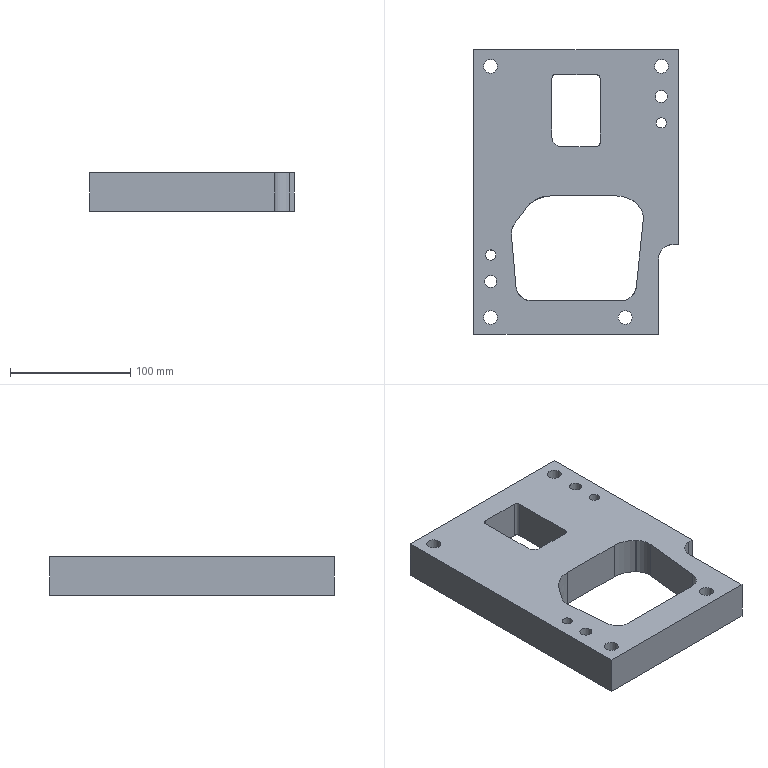Part | STEP file | lll_id3646_x_t | 1 solid | 45 faces | box 170 x 237 x 32 mm | volume 864357 mm3 | plane 22 | cylinder 19 | other 4 | commonest cylinder face diameters 11.509 x4 18.008 x4 6 x3 8.506 x2 10 x2 16 x1
STEP:
#1=CARTESIAN_POINT('',(3672.243,109.5,60.5));
#2=VERTEX_POINT('',#1);
#3=CARTESIAN_POINT('',(3668.,109.5,60.5));
#4=VERTEX_POINT('',#3);
#5=CARTESIAN_POINT('',(3700.5,109.5,60.5));
#6=DIRECTION('',(-1.,0.,0.));
#7=VECTOR('',#6,1.);
#8=LINE('',#5,#7);
#9=EDGE_CURVE('',#2,#4,#8,.T.);
#10=ORIENTED_EDGE('',*,*,#9,.T.);
#11=CARTESIAN_POINT('',(3656.,97.5,60.5));
#12=VERTEX_POINT('',#11);
#13=CARTESIAN_POINT('',(3668.,97.5,60.5));
#14=DIRECTION('',(0.,0.,1.));
#15=DIRECTION('',(-1.,0.,0.));
#16=AXIS2_PLACEMENT_3D('',#13,#14,#15);
#17=CIRCLE('',#16,12.);
#18=EDGE_CURVE('',#4,#12,#17,.T.);
#19=ORIENTED_EDGE('',*,*,#18,.T.);
#20=CARTESIAN_POINT('',(3656.,34.803,60.5));
#21=VERTEX_POINT('',#20);
#22=CARTESIAN_POINT('',(3656.,0.00007612,60.5));
#23=DIRECTION('',(0.,-1.,0.));
#24=VECTOR('',#23,1.);
#25=LINE('',#22,#24);
#26=EDGE_CURVE('',#12,#21,#25,.T.);
#27=ORIENTED_EDGE('',*,*,#26,.T.);
#28=CARTESIAN_POINT('',(3502.243,34.803,60.5));
#29=VERTEX_POINT('',#28);
#30=CARTESIAN_POINT('',(3587.243,34.803,60.5));
#31=DIRECTION('',(1.,0.,0.));
#32=VECTOR('',#31,1.);
#33=LINE('',#30,#32);
#34=EDGE_CURVE('',#29,#21,#33,.T.);
#35=ORIENTED_EDGE('',*,*,#34,.F.);
#36=CARTESIAN_POINT('',(3502.243,271.803,60.5));
#37=VERTEX_POINT('',#36);
#38=CARTESIAN_POINT('',(3502.243,156.803,60.5));
#39=DIRECTION('',(0.,-1.,0.));
#40=VECTOR('',#39,1.);
#41=LINE('',#38,#40);
#42=EDGE_CURVE('',#37,#29,#41,.T.);
#43=ORIENTED_EDGE('',*,*,#42,.F.);
#44=CARTESIAN_POINT('',(3672.243,271.803,60.5));
#45=VERTEX_POINT('',#44);
#46=CARTESIAN_POINT('',(3587.243,271.803,60.5));
#47=DIRECTION('',(-1.,0.,0.));
#48=VECTOR('',#47,1.);
#49=LINE('',#46,#48);
#50=EDGE_CURVE('',#45,#37,#49,.T.);
#51=ORIENTED_EDGE('',*,*,#50,.F.);
#52=CARTESIAN_POINT('',(3672.243,156.803,60.5));
#53=DIRECTION('',(0.,1.,0.));
#54=VECTOR('',#53,1.);
#55=LINE('',#52,#54);
#56=EDGE_CURVE('',#2,#45,#55,.T.);
#57=ORIENTED_EDGE('',*,*,#56,.F.);
#58=EDGE_LOOP('',(#10,#19,#27,#35,#43,#51,#57));
#59=FACE_BOUND('',#58,.T.);
#60=CARTESIAN_POINT('',(3511.99,100.803,60.5));
#61=VERTEX_POINT('',#60);
#62=CARTESIAN_POINT('',(3516.243,100.803,60.5));
#63=DIRECTION('',(0.,0.,1.));
#64=DIRECTION('',(-1.,0.,0.));
#65=AXIS2_PLACEMENT_3D('',#62,#63,#64);
#66=CIRCLE('',#65,4.253);
#67=EDGE_CURVE('',#61,#61,#66,.T.);
#68=ORIENTED_EDGE('',*,*,#67,.T.);
#69=EDGE_LOOP('',(#68));
#70=FACE_BOUND('',#69,.T.);
#71=CARTESIAN_POINT('',(3521.244,78.803,60.5));
#72=VERTEX_POINT('',#71);
#73=CARTESIAN_POINT('',(3516.243,78.803,60.5));
#74=DIRECTION('',(0.,0.,-1.));
#75=DIRECTION('',(1.,0.,0.));
#76=AXIS2_PLACEMENT_3D('',#73,#74,#75);
#77=CIRCLE('',#76,5.);
#78=EDGE_CURVE('',#72,#72,#77,.T.);
#79=ORIENTED_EDGE('',*,*,#78,.F.);
#80=EDGE_LOOP('',(#79));
#81=FACE_BOUND('',#80,.T.);
#82=CARTESIAN_POINT('',(3663.244,232.803,60.5));
#83=VERTEX_POINT('',#82);
#84=CARTESIAN_POINT('',(3658.243,232.803,60.5));
#85=DIRECTION('',(0.,0.,-1.));
#86=DIRECTION('',(1.,0.,0.));
#87=AXIS2_PLACEMENT_3D('',#84,#85,#86);
#88=CIRCLE('',#87,5.);
#89=EDGE_CURVE('',#83,#83,#88,.T.);
#90=ORIENTED_EDGE('',*,*,#89,.F.);
#91=EDGE_LOOP('',(#90));
#92=FACE_BOUND('',#91,.T.);
#93=CARTESIAN_POINT('',(3507.239,257.803,60.5));
#94=VERTEX_POINT('',#93);
#95=CARTESIAN_POINT('',(3516.243,257.803,60.5));
#96=DIRECTION('',(0.,0.,1.));
#97=DIRECTION('',(-1.,0.,0.));
#98=AXIS2_PLACEMENT_3D('',#95,#96,#97);
#99=CIRCLE('',#98,9.004);
#100=EDGE_CURVE('',#94,#94,#99,.T.);
#101=ORIENTED_EDGE('',*,*,#100,.T.);
#102=EDGE_LOOP('',(#101));
#103=FACE_BOUND('',#102,.T.);
#104=CARTESIAN_POINT('',(3649.239,257.803,60.5));
#105=VERTEX_POINT('',#104);
#106=CARTESIAN_POINT('',(3658.243,257.803,60.5));
#107=DIRECTION('',(0.,0.,1.));
#108=DIRECTION('',(-1.,0.,0.));
#109=AXIS2_PLACEMENT_3D('',#106,#107,#108);
#110=CIRCLE('',#109,9.004);
#111=EDGE_CURVE('',#105,#105,#110,.T.);
#112=ORIENTED_EDGE('',*,*,#111,.T.);
#113=EDGE_LOOP('',(#112));
#114=FACE_BOUND('',#113,.T.);
#115=CARTESIAN_POINT('',(3507.239,48.803,60.5));
#116=VERTEX_POINT('',#115);
#117=CARTESIAN_POINT('',(3516.243,48.803,60.5));
#118=DIRECTION('',(0.,0.,1.));
#119=DIRECTION('',(-1.,0.,0.));
#120=AXIS2_PLACEMENT_3D('',#117,#118,#119);
#121=CIRCLE('',#120,9.004);
#122=EDGE_CURVE('',#116,#116,#121,.T.);
#123=ORIENTED_EDGE('',*,*,#122,.T.);
#124=EDGE_LOOP('',(#123));
#125=FACE_BOUND('',#124,.T.);
#126=CARTESIAN_POINT('',(3619.239,48.803,60.5));
#127=VERTEX_POINT('',#126);
#128=CARTESIAN_POINT('',(3628.243,48.803,60.5));
#129=DIRECTION('',(0.,0.,1.));
#130=DIRECTION('',(-1.,0.,0.));
#131=AXIS2_PLACEMENT_3D('',#128,#129,#130);
#132=CIRCLE('',#131,9.004);
#133=EDGE_CURVE('',#127,#127,#132,.T.);
#134=ORIENTED_EDGE('',*,*,#133,.T.);
#135=EDGE_LOOP('',(#134));
#136=FACE_BOUND('',#135,.T.);
#137=CARTESIAN_POINT('',(3653.99,210.803,60.5));
#138=VERTEX_POINT('',#137);
#139=CARTESIAN_POINT('',(3658.243,210.803,60.5));
#140=DIRECTION('',(0.,0.,1.));
#141=DIRECTION('',(-1.,0.,0.));
#142=AXIS2_PLACEMENT_3D('',#139,#140,#141);
#143=CIRCLE('',#142,4.253);
#144=EDGE_CURVE('',#138,#138,#143,.T.);
#145=ORIENTED_EDGE('',*,*,#144,.T.);
#146=EDGE_LOOP('',(#145));
#147=FACE_BOUND('',#146,.T.);
#148=CARTESIAN_POINT('',(3567.234,198.95,60.5));
#149=VERTEX_POINT('',#148);
#150=CARTESIAN_POINT('',(3567.234,247.95,60.5));
#151=VERTEX_POINT('',#150);
#152=CARTESIAN_POINT('',(3567.234,199.225,60.5));
#153=DIRECTION('',(0.,1.,0.));
#154=VECTOR('',#153,1.);
#155=LINE('',#152,#154);
#156=EDGE_CURVE('',#149,#151,#155,.T.);
#157=ORIENTED_EDGE('',*,*,#156,.F.);
#158=CARTESIAN_POINT('',(3575.234,190.95,60.5));
#159=VERTEX_POINT('',#158);
#160=CARTESIAN_POINT('',(3575.234,198.95,60.5));
#161=DIRECTION('',(0.,0.,1.));
#162=DIRECTION('',(1.,0.,0.));
#163=AXIS2_PLACEMENT_3D('',#160,#161,#162);
#164=CIRCLE('',#163,8.);
#165=EDGE_CURVE('',#149,#159,#164,.T.);
#166=ORIENTED_EDGE('',*,*,#165,.T.);
#167=CARTESIAN_POINT('',(3604.234,190.95,60.5));
#168=VERTEX_POINT('',#167);
#169=CARTESIAN_POINT('',(3587.234,190.95,60.5));
#170=DIRECTION('',(-1.,0.,0.));
#171=VECTOR('',#170,1.);
#172=LINE('',#169,#171);
#173=EDGE_CURVE('',#168,#159,#172,.T.);
#174=ORIENTED_EDGE('',*,*,#173,.F.);
#175=CARTESIAN_POINT('',(3607.234,193.95,60.5));
#176=VERTEX_POINT('',#175);
#177=CARTESIAN_POINT('',(3604.234,193.95,60.5));
#178=DIRECTION('',(0.,0.,1.));
#179=DIRECTION('',(1.,0.,0.));
#180=AXIS2_PLACEMENT_3D('',#177,#178,#179);
#181=CIRCLE('',#180,3.);
#182=EDGE_CURVE('',#168,#176,#181,.T.);
#183=ORIENTED_EDGE('',*,*,#182,.T.);
#184=CARTESIAN_POINT('',(3607.234,247.95,60.5));
#185=VERTEX_POINT('',#184);
#186=CARTESIAN_POINT('',(3607.234,199.225,60.5));
#187=DIRECTION('',(0.,-1.,0.));
#188=VECTOR('',#187,1.);
#189=LINE('',#186,#188);
#190=EDGE_CURVE('',#185,#176,#189,.T.);
#191=ORIENTED_EDGE('',*,*,#190,.F.);
#192=CARTESIAN_POINT('',(3604.234,250.95,60.5));
#193=VERTEX_POINT('',#192);
#194=CARTESIAN_POINT('',(3604.234,247.95,60.5));
#195=DIRECTION('',(0.,0.,1.));
#196=DIRECTION('',(1.,0.,0.));
#197=AXIS2_PLACEMENT_3D('',#194,#195,#196);
#198=CIRCLE('',#197,3.);
#199=EDGE_CURVE('',#185,#193,#198,.T.);
#200=ORIENTED_EDGE('',*,*,#199,.T.);
#201=CARTESIAN_POINT('',(3570.234,250.95,60.5));
#202=VERTEX_POINT('',#201);
#203=CARTESIAN_POINT('',(3587.234,250.95,60.5));
#204=DIRECTION('',(1.,0.,0.));
#205=VECTOR('',#204,1.);
#206=LINE('',#203,#205);
#207=EDGE_CURVE('',#202,#193,#206,.T.);
#208=ORIENTED_EDGE('',*,*,#207,.F.);
#209=CARTESIAN_POINT('',(3570.234,247.95,60.5));
#210=DIRECTION('',(0.,0.,1.));
#211=DIRECTION('',(1.,0.,0.));
#212=AXIS2_PLACEMENT_3D('',#209,#210,#211);
#213=CIRCLE('',#212,3.);
#214=EDGE_CURVE('',#202,#151,#213,.T.);
#215=ORIENTED_EDGE('',*,*,#214,.T.);
#216=EDGE_LOOP('',(#157,#166,#174,#183,#191,#200,#208,#215));
#217=FACE_BOUND('',#216,.T.);
#218=CARTESIAN_POINT('',(3620.83,150.017,60.5));
#219=VERTEX_POINT('',#218);
#220=CARTESIAN_POINT('',(3638.507,142.694,60.5));
#221=VERTEX_POINT('',#220);
#222=CARTESIAN_POINT('',(3620.83,125.017,60.5));
#223=DIRECTION('',(0.,0.,-1.));
#224=DIRECTION('',(-1.,0.,0.));
#225=AXIS2_PLACEMENT_3D('',#222,#223,#224);
#226=CIRCLE('',#225,25.);
#227=EDGE_CURVE('',#219,#221,#226,.T.);
#228=ORIENTED_EDGE('',*,*,#227,.F.);
#229=CARTESIAN_POINT('',(3565.78,150.017,60.5));
#230=VERTEX_POINT('',#229);
#231=CARTESIAN_POINT('',(3587.243,150.017,60.5));
#232=DIRECTION('',(1.,0.,0.));
#233=VECTOR('',#232,1.);
#234=LINE('',#231,#233);
#235=EDGE_CURVE('',#230,#219,#234,.T.);
#236=ORIENTED_EDGE('',*,*,#235,.F.);
#237=CARTESIAN_POINT('',(3545.814,140.062,60.5));
#238=VERTEX_POINT('',#237);
#239=CARTESIAN_POINT('',(3545.814,140.062,60.5));
#240=CARTESIAN_POINT('',(3548.154,143.168,60.5));
#241=CARTESIAN_POINT('',(3551.201,145.685,60.5));
#242=CARTESIAN_POINT('',(3556.357,148.252,60.5));
#243=CARTESIAN_POINT('',(3558.2,148.927,60.5));
#244=CARTESIAN_POINT('',(3561.932,149.802,60.5));
#245=CARTESIAN_POINT('',(3563.837,150.017,60.5));
#246=CARTESIAN_POINT('',(3565.78,150.017,60.5));
#247=B_SPLINE_CURVE_WITH_KNOTS('',3,(#239,#240,#241,#242,#243,#244,#245,#246),.UNSPECIFIED.,.F.,.F.,(4,2,2,4),(0.,0.5,0.75,1.),.UNSPECIFIED.);
#248=EDGE_CURVE('',#238,#230,#247,.T.);
#249=ORIENTED_EDGE('',*,*,#248,.F.);
#250=CARTESIAN_POINT('',(3536.487,127.684,60.5));
#251=VERTEX_POINT('',#250);
#252=CARTESIAN_POINT('',(3568.865,170.652,60.5));
#253=DIRECTION('',(0.6018,0.7986,0.));
#254=VECTOR('',#253,1.);
#255=LINE('',#252,#254);
#256=EDGE_CURVE('',#251,#238,#255,.T.);
#257=ORIENTED_EDGE('',*,*,#256,.F.);
#258=CARTESIAN_POINT('',(3533.523,117.349,60.5));
#259=VERTEX_POINT('',#258);
#260=CARTESIAN_POINT('',(3533.523,117.349,60.5));
#261=CARTESIAN_POINT('',(3533.202,121.023,60.5));
#262=CARTESIAN_POINT('',(3534.267,124.739,60.5));
#263=CARTESIAN_POINT('',(3536.487,127.684,60.5));
#264=B_SPLINE_CURVE_WITH_KNOTS('',3,(#260,#261,#262,#263),.UNSPECIFIED.,.F.,.F.,(4,4),(0.,1.),.UNSPECIFIED.);
#265=EDGE_CURVE('',#259,#251,#264,.T.);
#266=ORIENTED_EDGE('',*,*,#265,.F.);
#267=CARTESIAN_POINT('',(3537.286,74.341,60.5));
#268=VERTEX_POINT('',#267);
#269=CARTESIAN_POINT('',(3530.506,151.839,60.5));
#270=DIRECTION('',(-0.08716,0.9962,0.));
#271=VECTOR('',#270,1.);
#272=LINE('',#269,#271);
#273=EDGE_CURVE('',#268,#259,#272,.T.);
#274=ORIENTED_EDGE('',*,*,#273,.F.);
#275=CARTESIAN_POINT('',(3550.037,62.657,60.5));
#276=VERTEX_POINT('',#275);
#277=CARTESIAN_POINT('',(3550.037,62.657,60.5));
#278=CARTESIAN_POINT('',(3546.846,62.657,60.5));
#279=CARTESIAN_POINT('',(3543.729,63.878,60.5));
#280=CARTESIAN_POINT('',(3539.06,68.152,60.5));
#281=CARTESIAN_POINT('',(3537.564,71.158,60.5));
#282=CARTESIAN_POINT('',(3537.286,74.341,60.5));
#283=B_SPLINE_CURVE_WITH_KNOTS('',3,(#277,#278,#279,#280,#281,#282),.UNSPECIFIED.,.F.,.F.,(4,2,4),(0.,0.5,1.),.UNSPECIFIED.);
#284=EDGE_CURVE('',#276,#268,#283,.T.);
#285=ORIENTED_EDGE('',*,*,#284,.F.);
#286=CARTESIAN_POINT('',(3624.637,62.657,60.5));
#287=VERTEX_POINT('',#286);
#288=CARTESIAN_POINT('',(3587.243,62.657,60.5));
#289=DIRECTION('',(-1.,0.,0.));
#290=VECTOR('',#289,1.);
#291=LINE('',#288,#290);
#292=EDGE_CURVE('',#287,#276,#291,.T.);
#293=ORIENTED_EDGE('',*,*,#292,.F.);
#294=CARTESIAN_POINT('',(3637.367,74.119,60.5));
#295=VERTEX_POINT('',#294);
#296=CARTESIAN_POINT('',(3637.367,74.119,60.5));
#297=CARTESIAN_POINT('',(3637.037,70.982,60.5));
#298=CARTESIAN_POINT('',(3635.532,68.044,60.5));
#299=CARTESIAN_POINT('',(3630.881,63.852,60.5));
#300=CARTESIAN_POINT('',(3627.795,62.657,60.5));
#301=CARTESIAN_POINT('',(3624.637,62.657,60.5));
#302=B_SPLINE_CURVE_WITH_KNOTS('',3,(#296,#297,#298,#299,#300,#301),.UNSPECIFIED.,.F.,.F.,(4,2,4),(0.,0.5,1.),.UNSPECIFIED.);
#303=EDGE_CURVE('',#295,#287,#302,.T.);
#304=ORIENTED_EDGE('',*,*,#303,.F.);
#305=CARTESIAN_POINT('',(3643.25,130.089,60.5));
#306=VERTEX_POINT('',#305);
#307=CARTESIAN_POINT('',(3645.415,150.689,60.5));
#308=DIRECTION('',(-0.1045,-0.9945,0.));
#309=VECTOR('',#308,1.);
#310=LINE('',#307,#309);
#311=EDGE_CURVE('',#306,#295,#310,.T.);
#312=ORIENTED_EDGE('',*,*,#311,.F.);
#313=CARTESIAN_POINT('',(3638.938,142.263,60.5));
#314=VERTEX_POINT('',#313);
#315=CARTESIAN_POINT('',(3628.332,131.657,60.5));
#316=DIRECTION('',(0.,0.,-1.));
#317=DIRECTION('',(-1.,0.,0.));
#318=AXIS2_PLACEMENT_3D('',#315,#316,#317);
#319=CIRCLE('',#318,15.);
#320=EDGE_CURVE('',#314,#306,#319,.T.);
#321=ORIENTED_EDGE('',*,*,#320,.F.);
#322=CARTESIAN_POINT('',(3605.821,175.381,60.5));
#323=DIRECTION('',(-0.7071,0.7071,0.));
#324=VECTOR('',#323,1.);
#325=LINE('',#322,#324);
#326=EDGE_CURVE('',#314,#221,#325,.T.);
#327=ORIENTED_EDGE('',*,*,#326,.T.);
#328=EDGE_LOOP('',(#228,#236,#249,#257,#266,#274,#285,#293,#304,#312,#321,#327));
#329=FACE_BOUND('',#328,.T.);
#330=CARTESIAN_POINT('',(3587.243,156.803,60.5));
#331=DIRECTION('',(0.,0.,-1.));
#332=DIRECTION('',(1.,0.,0.));
#333=AXIS2_PLACEMENT_3D('',#330,#331,#332);
#334=PLANE('',#333);
#335=ADVANCED_FACE('',(#59,#70,#81,#92,#103,#114,#125,#136,#147,#217,#329),#334,.T.);
#336=CARTESIAN_POINT('',(3656.,34.803,92.5));
#337=VERTEX_POINT('',#336);
#338=CARTESIAN_POINT('',(3656.,97.5,92.5));
#339=VERTEX_POINT('',#338);
#340=CARTESIAN_POINT('',(3656.,0.00007612,92.5));
#341=DIRECTION('',(0.,1.,0.));
#342=VECTOR('',#341,1.);
#343=LINE('',#340,#342);
#344=EDGE_CURVE('',#337,#339,#343,.T.);
#345=ORIENTED_EDGE('',*,*,#344,.T.);
#346=CARTESIAN_POINT('',(3668.,109.5,92.5));
#347=VERTEX_POINT('',#346);
#348=CARTESIAN_POINT('',(3668.,97.5,92.5));
#349=DIRECTION('',(0.,0.,-1.));
#350=DIRECTION('',(1.,0.,0.));
#351=AXIS2_PLACEMENT_3D('',#348,#349,#350);
#352=CIRCLE('',#351,12.);
#353=EDGE_CURVE('',#339,#347,#352,.T.);
#354=ORIENTED_EDGE('',*,*,#353,.T.);
#355=CARTESIAN_POINT('',(3672.243,109.5,92.5));
#356=VERTEX_POINT('',#355);
#357=CARTESIAN_POINT('',(3700.5,109.5,92.5));
#358=DIRECTION('',(1.,0.,0.));
#359=VECTOR('',#358,1.);
#360=LINE('',#357,#359);
#361=EDGE_CURVE('',#347,#356,#360,.T.);
#362=ORIENTED_EDGE('',*,*,#361,.T.);
#363=CARTESIAN_POINT('',(3672.243,271.803,92.5));
#364=VERTEX_POINT('',#363);
#365=CARTESIAN_POINT('',(3672.243,156.803,92.5));
#366=DIRECTION('',(0.,-1.,0.));
#367=VECTOR('',#366,1.);
#368=LINE('',#365,#367);
#369=EDGE_CURVE('',#364,#356,#368,.T.);
#370=ORIENTED_EDGE('',*,*,#369,.F.);
#371=CARTESIAN_POINT('',(3502.243,271.803,92.5));
#372=VERTEX_POINT('',#371);
#373=CARTESIAN_POINT('',(3587.243,271.803,92.5));
#374=DIRECTION('',(1.,0.,0.));
#375=VECTOR('',#374,1.);
#376=LINE('',#373,#375);
#377=EDGE_CURVE('',#372,#364,#376,.T.);
#378=ORIENTED_EDGE('',*,*,#377,.F.);
#379=CARTESIAN_POINT('',(3502.243,34.803,92.5));
#380=VERTEX_POINT('',#379);
#381=CARTESIAN_POINT('',(3502.243,156.803,92.5));
#382=DIRECTION('',(0.,1.,0.));
#383=VECTOR('',#382,1.);
#384=LINE('',#381,#383);
#385=EDGE_CURVE('',#380,#372,#384,.T.);
#386=ORIENTED_EDGE('',*,*,#385,.F.);
#387=CARTESIAN_POINT('',(3587.243,34.803,92.5));
#388=DIRECTION('',(-1.,0.,0.));
#389=VECTOR('',#388,1.);
#390=LINE('',#387,#389);
#391=EDGE_CURVE('',#337,#380,#390,.T.);
#392=ORIENTED_EDGE('',*,*,#391,.F.);
#393=EDGE_LOOP('',(#345,#354,#362,#370,#378,#386,#392));
#394=FACE_BOUND('',#393,.T.);
#395=CARTESIAN_POINT('',(3653.99,210.803,92.5));
#396=VERTEX_POINT('',#395);
#397=CARTESIAN_POINT('',(3658.243,210.803,92.5));
#398=DIRECTION('',(0.,0.,1.));
#399=DIRECTION('',(-1.,0.,0.));
#400=AXIS2_PLACEMENT_3D('',#397,#398,#399);
#401=CIRCLE('',#400,4.253);
#402=EDGE_CURVE('',#396,#396,#401,.T.);
#403=ORIENTED_EDGE('',*,*,#402,.F.);
#404=EDGE_LOOP('',(#403));
#405=FACE_BOUND('',#404,.T.);
#406=CARTESIAN_POINT('',(3511.99,100.803,92.5));
#407=VERTEX_POINT('',#406);
#408=CARTESIAN_POINT('',(3516.243,100.803,92.5));
#409=DIRECTION('',(0.,0.,1.));
#410=DIRECTION('',(-1.,0.,0.));
#411=AXIS2_PLACEMENT_3D('',#408,#409,#410);
#412=CIRCLE('',#411,4.253);
#413=EDGE_CURVE('',#407,#407,#412,.T.);
#414=ORIENTED_EDGE('',*,*,#413,.F.);
#415=EDGE_LOOP('',(#414));
#416=FACE_BOUND('',#415,.T.);
#417=CARTESIAN_POINT('',(3511.243,78.803,92.5));
#418=VERTEX_POINT('',#417);
#419=CARTESIAN_POINT('',(3516.243,78.803,92.5));
#420=DIRECTION('',(0.,0.,1.));
#421=DIRECTION('',(-1.,0.,0.));
#422=AXIS2_PLACEMENT_3D('',#419,#420,#421);
#423=CIRCLE('',#422,5.);
#424=EDGE_CURVE('',#418,#418,#423,.T.);
#425=ORIENTED_EDGE('',*,*,#424,.F.);
#426=EDGE_LOOP('',(#425));
#427=FACE_BOUND('',#426,.T.);
#428=CARTESIAN_POINT('',(3653.243,232.803,92.5));
#429=VERTEX_POINT('',#428);
#430=CARTESIAN_POINT('',(3658.243,232.803,92.5));
#431=DIRECTION('',(0.,0.,1.));
#432=DIRECTION('',(-1.,0.,0.));
#433=AXIS2_PLACEMENT_3D('',#430,#431,#432);
#434=CIRCLE('',#433,5.);
#435=EDGE_CURVE('',#429,#429,#434,.T.);
#436=ORIENTED_EDGE('',*,*,#435,.F.);
#437=EDGE_LOOP('',(#436));
#438=FACE_BOUND('',#437,.T.);
#439=CARTESIAN_POINT('',(3622.489,48.803,92.5));
#440=VERTEX_POINT('',#439);
#441=CARTESIAN_POINT('',(3628.243,48.803,92.5));
#442=DIRECTION('',(0.,0.,1.));
#443=DIRECTION('',(-1.,0.,0.));
#444=AXIS2_PLACEMENT_3D('',#441,#442,#443);
#445=CIRCLE('',#444,5.755);
#446=EDGE_CURVE('',#440,#440,#445,.T.);
#447=ORIENTED_EDGE('',*,*,#446,.F.);
#448=EDGE_LOOP('',(#447));
#449=FACE_BOUND('',#448,.T.);
#450=CARTESIAN_POINT('',(3510.489,257.803,92.5));
#451=VERTEX_POINT('',#450);
#452=CARTESIAN_POINT('',(3516.243,257.803,92.5));
#453=DIRECTION('',(0.,0.,1.));
#454=DIRECTION('',(-1.,0.,0.));
#455=AXIS2_PLACEMENT_3D('',#452,#453,#454);
#456=CIRCLE('',#455,5.755);
#457=EDGE_CURVE('',#451,#451,#456,.T.);
#458=ORIENTED_EDGE('',*,*,#457,.F.);
#459=EDGE_LOOP('',(#458));
#460=FACE_BOUND('',#459,.T.);
#461=CARTESIAN_POINT('',(3510.489,48.803,92.5));
#462=VERTEX_POINT('',#461);
#463=CARTESIAN_POINT('',(3516.243,48.803,92.5));
#464=DIRECTION('',(0.,0.,1.));
#465=DIRECTION('',(-1.,0.,0.));
#466=AXIS2_PLACEMENT_3D('',#463,#464,#465);
#467=CIRCLE('',#466,5.755);
#468=EDGE_CURVE('',#462,#462,#467,.T.);
#469=ORIENTED_EDGE('',*,*,#468,.F.);
#470=EDGE_LOOP('',(#469));
#471=FACE_BOUND('',#470,.T.);
#472=CARTESIAN_POINT('',(3652.489,257.803,92.5));
#473=VERTEX_POINT('',#472);
#474=CARTESIAN_POINT('',(3658.243,257.803,92.5));
#475=DIRECTION('',(0.,0.,1.));
#476=DIRECTION('',(-1.,0.,0.));
#477=AXIS2_PLACEMENT_3D('',#474,#475,#476);
#478=CIRCLE('',#477,5.755);
#479=EDGE_CURVE('',#473,#473,#478,.T.);
#480=ORIENTED_EDGE('',*,*,#479,.F.);
#481=EDGE_LOOP('',(#480));
#482=FACE_BOUND('',#481,.T.);
#483=CARTESIAN_POINT('',(3575.234,190.95,92.5));
#484=VERTEX_POINT('',#483);
#485=CARTESIAN_POINT('',(3604.234,190.95,92.5));
#486=VERTEX_POINT('',#485);
#487=CARTESIAN_POINT('',(3587.234,190.95,92.5));
#488=DIRECTION('',(1.,0.,0.));
#489=VECTOR('',#488,1.);
#490=LINE('',#487,#489);
#491=EDGE_CURVE('',#484,#486,#490,.T.);
#492=ORIENTED_EDGE('',*,*,#491,.F.);
#493=CARTESIAN_POINT('',(3567.234,198.95,92.5));
#494=VERTEX_POINT('',#493);
#495=CARTESIAN_POINT('',(3575.234,198.95,92.5));
#496=DIRECTION('',(0.,0.,-1.));
#497=DIRECTION('',(-1.,0.,0.));
#498=AXIS2_PLACEMENT_3D('',#495,#496,#497);
#499=CIRCLE('',#498,8.);
#500=EDGE_CURVE('',#484,#494,#499,.T.);
#501=ORIENTED_EDGE('',*,*,#500,.T.);
#502=CARTESIAN_POINT('',(3567.234,247.95,92.5));
#503=VERTEX_POINT('',#502);
#504=CARTESIAN_POINT('',(3567.234,199.225,92.5));
#505=DIRECTION('',(0.,-1.,0.));
#506=VECTOR('',#505,1.);
#507=LINE('',#504,#506);
#508=EDGE_CURVE('',#503,#494,#507,.T.);
#509=ORIENTED_EDGE('',*,*,#508,.F.);
#510=CARTESIAN_POINT('',(3570.234,250.95,92.5));
#511=VERTEX_POINT('',#510);
#512=CARTESIAN_POINT('',(3570.234,247.95,92.5));
#513=DIRECTION('',(0.,0.,-1.));
#514=DIRECTION('',(-1.,0.,0.));
#515=AXIS2_PLACEMENT_3D('',#512,#513,#514);
#516=CIRCLE('',#515,3.);
#517=EDGE_CURVE('',#503,#511,#516,.T.);
#518=ORIENTED_EDGE('',*,*,#517,.T.);
#519=CARTESIAN_POINT('',(3604.234,250.95,92.5));
#520=VERTEX_POINT('',#519);
#521=CARTESIAN_POINT('',(3587.234,250.95,92.5));
#522=DIRECTION('',(-1.,0.,0.));
#523=VECTOR('',#522,1.);
#524=LINE('',#521,#523);
#525=EDGE_CURVE('',#520,#511,#524,.T.);
#526=ORIENTED_EDGE('',*,*,#525,.F.);
#527=CARTESIAN_POINT('',(3607.234,247.95,92.5));
#528=VERTEX_POINT('',#527);
#529=CARTESIAN_POINT('',(3604.234,247.95,92.5));
#530=DIRECTION('',(0.,0.,-1.));
#531=DIRECTION('',(-1.,0.,0.));
#532=AXIS2_PLACEMENT_3D('',#529,#530,#531);
#533=CIRCLE('',#532,3.);
#534=EDGE_CURVE('',#520,#528,#533,.T.);
#535=ORIENTED_EDGE('',*,*,#534,.T.);
#536=CARTESIAN_POINT('',(3607.234,193.95,92.5));
#537=VERTEX_POINT('',#536);
#538=CARTESIAN_POINT('',(3607.234,199.225,92.5));
#539=DIRECTION('',(0.,1.,0.));
#540=VECTOR('',#539,1.);
#541=LINE('',#538,#540);
#542=EDGE_CURVE('',#537,#528,#541,.T.);
#543=ORIENTED_EDGE('',*,*,#542,.F.);
#544=CARTESIAN_POINT('',(3604.234,193.95,92.5));
#545=DIRECTION('',(0.,0.,-1.));
#546=DIRECTION('',(-1.,0.,0.));
#547=AXIS2_PLACEMENT_3D('',#544,#545,#546);
#548=CIRCLE('',#547,3.);
#549=EDGE_CURVE('',#537,#486,#548,.T.);
#550=ORIENTED_EDGE('',*,*,#549,.T.);
#551=EDGE_LOOP('',(#492,#501,#509,#518,#526,#535,#543,#550));
#552=FACE_BOUND('',#551,.T.);
#553=CARTESIAN_POINT('',(3643.25,130.089,92.5));
#554=VERTEX_POINT('',#553);
#555=CARTESIAN_POINT('',(3638.938,142.263,92.5));
#556=VERTEX_POINT('',#555);
#557=CARTESIAN_POINT('',(3628.332,131.657,92.5));
#558=DIRECTION('',(0.,0.,1.));
#559=DIRECTION('',(1.,0.,0.));
#560=AXIS2_PLACEMENT_3D('',#557,#558,#559);
#561=CIRCLE('',#560,15.);
#562=EDGE_CURVE('',#554,#556,#561,.T.);
#563=ORIENTED_EDGE('',*,*,#562,.F.);
#564=CARTESIAN_POINT('',(3637.367,74.119,92.5));
#565=VERTEX_POINT('',#564);
#566=CARTESIAN_POINT('',(3645.415,150.689,92.5));
#567=DIRECTION('',(0.1045,0.9945,0.));
#568=VECTOR('',#567,1.);
#569=LINE('',#566,#568);
#570=EDGE_CURVE('',#565,#554,#569,.T.);
#571=ORIENTED_EDGE('',*,*,#570,.F.);
#572=CARTESIAN_POINT('',(3624.637,62.657,92.5));
#573=VERTEX_POINT('',#572);
#574=CARTESIAN_POINT('',(3624.637,62.657,92.5));
#575=CARTESIAN_POINT('',(3627.791,62.657,92.5));
#576=CARTESIAN_POINT('',(3630.87,63.846,92.5));
#577=CARTESIAN_POINT('',(3635.525,68.034,92.5));
#578=CARTESIAN_POINT('',(3637.037,70.978,92.5));
#579=CARTESIAN_POINT('',(3637.367,74.119,92.5));
#580=B_SPLINE_CURVE_WITH_KNOTS('',3,(#574,#575,#576,#577,#578,#579),.UNSPECIFIED.,.F.,.F.,(4,2,4),(0.,0.5,1.),.UNSPECIFIED.);
#581=EDGE_CURVE('',#573,#565,#580,.T.);
#582=ORIENTED_EDGE('',*,*,#581,.F.);
#583=CARTESIAN_POINT('',(3550.037,62.657,92.5));
#584=VERTEX_POINT('',#583);
#585=CARTESIAN_POINT('',(3587.243,62.657,92.5));
#586=DIRECTION('',(1.,0.,0.));
#587=VECTOR('',#586,1.);
#588=LINE('',#585,#587);
#589=EDGE_CURVE('',#584,#573,#588,.T.);
#590=ORIENTED_EDGE('',*,*,#589,.F.);
#591=CARTESIAN_POINT('',(3537.286,74.341,92.5));
#592=VERTEX_POINT('',#591);
#593=CARTESIAN_POINT('',(3537.286,74.341,92.5));
#594=CARTESIAN_POINT('',(3537.564,71.162,92.5));
#595=CARTESIAN_POINT('',(3539.052,68.163,92.5));
#596=CARTESIAN_POINT('',(3543.717,63.885,92.5));
#597=CARTESIAN_POINT('',(3546.842,62.657,92.5));
#598=CARTESIAN_POINT('',(3550.037,62.657,92.5));
#599=B_SPLINE_CURVE_WITH_KNOTS('',3,(#593,#594,#595,#596,#597,#598),.UNSPECIFIED.,.F.,.F.,(4,2,4),(0.,0.5,1.),.UNSPECIFIED.);
#600=EDGE_CURVE('',#592,#584,#599,.T.);
#601=ORIENTED_EDGE('',*,*,#600,.F.);
#602=CARTESIAN_POINT('',(3533.523,117.349,92.5));
#603=VERTEX_POINT('',#602);
#604=CARTESIAN_POINT('',(3530.506,151.839,92.5));
#605=DIRECTION('',(0.08716,-0.9962,0.));
#606=VECTOR('',#605,1.);
#607=LINE('',#604,#606);
#608=EDGE_CURVE('',#603,#592,#607,.T.);
#609=ORIENTED_EDGE('',*,*,#608,.F.);
#610=CARTESIAN_POINT('',(3536.487,127.684,92.5));
#611=VERTEX_POINT('',#610);
#612=CARTESIAN_POINT('',(3536.487,127.684,92.5));
#613=CARTESIAN_POINT('',(3534.267,124.738,92.5));
#614=CARTESIAN_POINT('',(3533.202,121.023,92.5));
#615=CARTESIAN_POINT('',(3533.523,117.349,92.5));
#616=B_SPLINE_CURVE_WITH_KNOTS('',3,(#612,#613,#614,#615),.UNSPECIFIED.,.F.,.F.,(4,4),(0.,1.),.UNSPECIFIED.);
#617=EDGE_CURVE('',#611,#603,#616,.T.);
#618=ORIENTED_EDGE('',*,*,#617,.F.);
#619=CARTESIAN_POINT('',(3545.814,140.062,92.5));
#620=VERTEX_POINT('',#619);
#621=CARTESIAN_POINT('',(3568.865,170.652,92.5));
#622=DIRECTION('',(-0.6018,-0.7986,0.));
#623=VECTOR('',#622,1.);
#624=LINE('',#621,#623);
#625=EDGE_CURVE('',#620,#611,#624,.T.);
#626=ORIENTED_EDGE('',*,*,#625,.F.);
#627=CARTESIAN_POINT('',(3565.78,150.017,92.5));
#628=VERTEX_POINT('',#627);
#629=CARTESIAN_POINT('',(3565.78,150.017,92.5));
#630=CARTESIAN_POINT('',(3561.891,150.017,92.5));
#631=CARTESIAN_POINT('',(3558.048,149.099,92.5));
#632=CARTESIAN_POINT('',(3552.894,146.526,92.5));
#633=CARTESIAN_POINT('',(3551.246,145.459,92.5));
#634=CARTESIAN_POINT('',(3548.301,143.006,92.5));
#635=CARTESIAN_POINT('',(3546.983,141.614,92.5));
#636=CARTESIAN_POINT('',(3545.814,140.062,92.5));
#637=B_SPLINE_CURVE_WITH_KNOTS('',3,(#629,#630,#631,#632,#633,#634,#635,#636),.UNSPECIFIED.,.F.,.F.,(4,2,2,4),(0.,0.5,0.75,1.),.UNSPECIFIED.);
#638=EDGE_CURVE('',#628,#620,#637,.T.);
#639=ORIENTED_EDGE('',*,*,#638,.F.);
#640=CARTESIAN_POINT('',(3620.83,150.017,92.5));
#641=VERTEX_POINT('',#640);
#642=CARTESIAN_POINT('',(3587.243,150.017,92.5));
#643=DIRECTION('',(-1.,0.,0.));
#644=VECTOR('',#643,1.);
#645=LINE('',#642,#644);
#646=EDGE_CURVE('',#641,#628,#645,.T.);
#647=ORIENTED_EDGE('',*,*,#646,.F.);
#648=CARTESIAN_POINT('',(3638.507,142.694,92.5));
#649=VERTEX_POINT('',#648);
#650=CARTESIAN_POINT('',(3620.83,125.017,92.5));
#651=DIRECTION('',(0.,0.,1.));
#652=DIRECTION('',(1.,0.,0.));
#653=AXIS2_PLACEMENT_3D('',#650,#651,#652);
#654=CIRCLE('',#653,25.);
#655=EDGE_CURVE('',#649,#641,#654,.T.);
#656=ORIENTED_EDGE('',*,*,#655,.F.);
#657=CARTESIAN_POINT('',(3565.868,215.334,92.5));
#658=DIRECTION('',(0.7071,-0.7071,0.));
#659=VECTOR('',#658,1.);
#660=LINE('',#657,#659);
#661=EDGE_CURVE('',#649,#556,#660,.T.);
#662=ORIENTED_EDGE('',*,*,#661,.T.);
#663=EDGE_LOOP('',(#563,#571,#582,#590,#601,#609,#618,#626,#639,#647,#656,#662));
#664=FACE_BOUND('',#663,.T.);
#665=CARTESIAN_POINT('',(3587.243,156.803,92.5));
#666=DIRECTION('',(0.,0.,1.));
#667=DIRECTION('',(-1.,0.,0.));
#668=AXIS2_PLACEMENT_3D('',#665,#666,#667);
#669=PLANE('',#668);
#670=ADVANCED_FACE('',(#394,#405,#416,#427,#438,#449,#460,#471,#482,#552,#664),#669,.T.);
#671=CARTESIAN_POINT('',(3672.243,109.5,60.5));
#672=DIRECTION('',(0.,0.,1.));
#673=VECTOR('',#672,1.);
#674=LINE('',#671,#673);
#675=EDGE_CURVE('',#2,#356,#674,.T.);
#676=ORIENTED_EDGE('',*,*,#675,.F.);
#677=ORIENTED_EDGE('',*,*,#56,.T.);
#678=CARTESIAN_POINT('',(3672.243,271.803,60.5));
#679=DIRECTION('',(0.,0.,1.));
#680=VECTOR('',#679,1.);
#681=LINE('',#678,#680);
#682=EDGE_CURVE('',#45,#364,#681,.T.);
#683=ORIENTED_EDGE('',*,*,#682,.T.);
#684=ORIENTED_EDGE('',*,*,#369,.T.);
#685=EDGE_LOOP('',(#676,#677,#683,#684));
#686=FACE_OUTER_BOUND('',#685,.T.);
#687=CARTESIAN_POINT('',(3672.243,156.803,60.5));
#688=DIRECTION('',(1.,0.,0.));
#689=DIRECTION('',(0.,0.,1.));
#690=AXIS2_PLACEMENT_3D('',#687,#688,#689);
#691=PLANE('',#690);
#692=ADVANCED_FACE('',(#686),#691,.T.);
#693=CARTESIAN_POINT('',(3502.243,271.803,60.5));
#694=DIRECTION('',(0.,0.,1.));
#695=VECTOR('',#694,1.);
#696=LINE('',#693,#695);
#697=EDGE_CURVE('',#37,#372,#696,.T.);
#698=ORIENTED_EDGE('',*,*,#697,.T.);
#699=ORIENTED_EDGE('',*,*,#377,.T.);
#700=ORIENTED_EDGE('',*,*,#682,.F.);
#701=ORIENTED_EDGE('',*,*,#50,.T.);
#702=EDGE_LOOP('',(#698,#699,#700,#701));
#703=FACE_OUTER_BOUND('',#702,.T.);
#704=CARTESIAN_POINT('',(3587.243,271.803,60.5));
#705=DIRECTION('',(0.,1.,0.));
#706=DIRECTION('',(0.,0.,-1.));
#707=AXIS2_PLACEMENT_3D('',#704,#705,#706);
#708=PLANE('',#707);
#709=ADVANCED_FACE('',(#703),#708,.T.);
#710=CARTESIAN_POINT('',(3656.,34.803,60.5));
#711=DIRECTION('',(0.,0.,-1.));
#712=VECTOR('',#711,1.);
#713=LINE('',#710,#712);
#714=EDGE_CURVE('',#337,#21,#713,.T.);
#715=ORIENTED_EDGE('',*,*,#714,.F.);
#716=ORIENTED_EDGE('',*,*,#391,.T.);
#717=CARTESIAN_POINT('',(3502.243,34.803,60.5));
#718=DIRECTION('',(0.,0.,1.));
#719=VECTOR('',#718,1.);
#720=LINE('',#717,#719);
#721=EDGE_CURVE('',#29,#380,#720,.T.);
#722=ORIENTED_EDGE('',*,*,#721,.F.);
#723=ORIENTED_EDGE('',*,*,#34,.T.);
#724=EDGE_LOOP('',(#715,#716,#722,#723));
#725=FACE_OUTER_BOUND('',#724,.T.);
#726=CARTESIAN_POINT('',(3587.243,34.803,60.5));
#727=DIRECTION('',(0.,-1.,0.));
#728=DIRECTION('',(0.,0.,1.));
#729=AXIS2_PLACEMENT_3D('',#726,#727,#728);
#730=PLANE('',#729);
#731=ADVANCED_FACE('',(#725),#730,.T.);
#732=ORIENTED_EDGE('',*,*,#42,.T.);
#733=ORIENTED_EDGE('',*,*,#721,.T.);
#734=ORIENTED_EDGE('',*,*,#385,.T.);
#735=ORIENTED_EDGE('',*,*,#697,.F.);
#736=EDGE_LOOP('',(#732,#733,#734,#735));
#737=FACE_OUTER_BOUND('',#736,.T.);
#738=CARTESIAN_POINT('',(3502.243,156.803,60.5));
#739=DIRECTION('',(-1.,0.,0.));
#740=DIRECTION('',(0.,0.,-1.));
#741=AXIS2_PLACEMENT_3D('',#738,#739,#740);
#742=PLANE('',#741);
#743=ADVANCED_FACE('',(#737),#742,.T.);
#744=ORIENTED_EDGE('',*,*,#479,.T.);
#745=EDGE_LOOP('',(#744));
#746=FACE_BOUND('',#745,.T.);
#747=CARTESIAN_POINT('',(3652.489,257.803,73.5));
#748=VERTEX_POINT('',#747);
#749=CARTESIAN_POINT('',(3658.243,257.803,73.5));
#750=DIRECTION('',(0.,0.,1.));
#751=DIRECTION('',(-1.,0.,0.));
#752=AXIS2_PLACEMENT_3D('',#749,#750,#751);
#753=CIRCLE('',#752,5.755);
#754=EDGE_CURVE('',#748,#748,#753,.T.);
#755=ORIENTED_EDGE('',*,*,#754,.F.);
#756=EDGE_LOOP('',(#755));
#757=FACE_BOUND('',#756,.T.);
#758=CARTESIAN_POINT('',(3658.243,257.803,57.5));
#759=DIRECTION('',(0.,0.,1.));
#760=DIRECTION('',(-1.,0.,0.));
#761=AXIS2_PLACEMENT_3D('',#758,#759,#760);
#762=CYLINDRICAL_SURFACE('',#761,5.755);
#763=ADVANCED_FACE('',(#746,#757),#762,.F.);
#764=ORIENTED_EDGE('',*,*,#754,.T.);
#765=EDGE_LOOP('',(#764));
#766=FACE_BOUND('',#765,.T.);
#767=CARTESIAN_POINT('',(3649.239,257.803,73.5));
#768=VERTEX_POINT('',#767);
#769=CARTESIAN_POINT('',(3658.243,257.803,73.5));
#770=DIRECTION('',(0.,0.,1.));
#771=DIRECTION('',(-1.,0.,0.));
#772=AXIS2_PLACEMENT_3D('',#769,#770,#771);
#773=CIRCLE('',#772,9.004);
#774=EDGE_CURVE('',#768,#768,#773,.T.);
#775=ORIENTED_EDGE('',*,*,#774,.F.);
#776=EDGE_LOOP('',(#775));
#777=FACE_BOUND('',#776,.T.);
#778=CARTESIAN_POINT('',(3658.243,257.803,73.5));
#779=DIRECTION('',(0.,0.,1.));
#780=DIRECTION('',(-1.,0.,0.));
#781=AXIS2_PLACEMENT_3D('',#778,#779,#780);
#782=PLANE('',#781);
#783=ADVANCED_FACE('',(#766,#777),#782,.F.);
#784=ORIENTED_EDGE('',*,*,#774,.T.);
#785=EDGE_LOOP('',(#784));
#786=FACE_BOUND('',#785,.T.);
#787=ORIENTED_EDGE('',*,*,#111,.F.);
#788=EDGE_LOOP('',(#787));
#789=FACE_BOUND('',#788,.T.);
#790=CARTESIAN_POINT('',(3658.243,257.803,60.5));
#791=DIRECTION('',(0.,0.,1.));
#792=DIRECTION('',(-1.,0.,0.));
#793=AXIS2_PLACEMENT_3D('',#790,#791,#792);
#794=CYLINDRICAL_SURFACE('',#793,9.004);
#795=ADVANCED_FACE('',(#786,#789),#794,.F.);
#796=ORIENTED_EDGE('',*,*,#468,.T.);
#797=EDGE_LOOP('',(#796));
#798=FACE_BOUND('',#797,.T.);
#799=CARTESIAN_POINT('',(3510.489,48.803,73.5));
#800=VERTEX_POINT('',#799);
#801=CARTESIAN_POINT('',(3516.243,48.803,73.5));
#802=DIRECTION('',(0.,0.,1.));
#803=DIRECTION('',(-1.,0.,0.));
#804=AXIS2_PLACEMENT_3D('',#801,#802,#803);
#805=CIRCLE('',#804,5.755);
#806=EDGE_CURVE('',#800,#800,#805,.T.);
#807=ORIENTED_EDGE('',*,*,#806,.F.);
#808=EDGE_LOOP('',(#807));
#809=FACE_BOUND('',#808,.T.);
#810=CARTESIAN_POINT('',(3516.243,48.803,57.5));
#811=DIRECTION('',(0.,0.,1.));
#812=DIRECTION('',(-1.,0.,0.));
#813=AXIS2_PLACEMENT_3D('',#810,#811,#812);
#814=CYLINDRICAL_SURFACE('',#813,5.755);
#815=ADVANCED_FACE('',(#798,#809),#814,.F.);
#816=ORIENTED_EDGE('',*,*,#806,.T.);
#817=EDGE_LOOP('',(#816));
#818=FACE_BOUND('',#817,.T.);
#819=CARTESIAN_POINT('',(3507.239,48.803,73.5));
#820=VERTEX_POINT('',#819);
#821=CARTESIAN_POINT('',(3516.243,48.803,73.5));
#822=DIRECTION('',(0.,0.,1.));
#823=DIRECTION('',(-1.,0.,0.));
#824=AXIS2_PLACEMENT_3D('',#821,#822,#823);
#825=CIRCLE('',#824,9.004);
#826=EDGE_CURVE('',#820,#820,#825,.T.);
#827=ORIENTED_EDGE('',*,*,#826,.F.);
#828=EDGE_LOOP('',(#827));
#829=FACE_BOUND('',#828,.T.);
#830=CARTESIAN_POINT('',(3516.243,48.803,73.5));
#831=DIRECTION('',(0.,0.,1.));
#832=DIRECTION('',(-1.,0.,0.));
#833=AXIS2_PLACEMENT_3D('',#830,#831,#832);
#834=PLANE('',#833);
#835=ADVANCED_FACE('',(#818,#829),#834,.F.);
#836=ORIENTED_EDGE('',*,*,#826,.T.);
#837=EDGE_LOOP('',(#836));
#838=FACE_BOUND('',#837,.T.);
#839=ORIENTED_EDGE('',*,*,#122,.F.);
#840=EDGE_LOOP('',(#839));
#841=FACE_BOUND('',#840,.T.);
#842=CARTESIAN_POINT('',(3516.243,48.803,60.5));
#843=DIRECTION('',(0.,0.,1.));
#844=DIRECTION('',(-1.,0.,0.));
#845=AXIS2_PLACEMENT_3D('',#842,#843,#844);
#846=CYLINDRICAL_SURFACE('',#845,9.004);
#847=ADVANCED_FACE('',(#838,#841),#846,.F.);
#848=ORIENTED_EDGE('',*,*,#457,.T.);
#849=EDGE_LOOP('',(#848));
#850=FACE_BOUND('',#849,.T.);
#851=CARTESIAN_POINT('',(3510.489,257.803,73.5));
#852=VERTEX_POINT('',#851);
#853=CARTESIAN_POINT('',(3516.243,257.803,73.5));
#854=DIRECTION('',(0.,0.,1.));
#855=DIRECTION('',(-1.,0.,0.));
#856=AXIS2_PLACEMENT_3D('',#853,#854,#855);
#857=CIRCLE('',#856,5.755);
#858=EDGE_CURVE('',#852,#852,#857,.T.);
#859=ORIENTED_EDGE('',*,*,#858,.F.);
#860=EDGE_LOOP('',(#859));
#861=FACE_BOUND('',#860,.T.);
#862=CARTESIAN_POINT('',(3516.243,257.803,57.5));
#863=DIRECTION('',(0.,0.,1.));
#864=DIRECTION('',(-1.,0.,0.));
#865=AXIS2_PLACEMENT_3D('',#862,#863,#864);
#866=CYLINDRICAL_SURFACE('',#865,5.755);
#867=ADVANCED_FACE('',(#850,#861),#866,.F.);
#868=ORIENTED_EDGE('',*,*,#858,.T.);
#869=EDGE_LOOP('',(#868));
#870=FACE_BOUND('',#869,.T.);
#871=CARTESIAN_POINT('',(3507.239,257.803,73.5));
#872=VERTEX_POINT('',#871);
#873=CARTESIAN_POINT('',(3516.243,257.803,73.5));
#874=DIRECTION('',(0.,0.,1.));
#875=DIRECTION('',(-1.,0.,0.));
#876=AXIS2_PLACEMENT_3D('',#873,#874,#875);
#877=CIRCLE('',#876,9.004);
#878=EDGE_CURVE('',#872,#872,#877,.T.);
#879=ORIENTED_EDGE('',*,*,#878,.F.);
#880=EDGE_LOOP('',(#879));
#881=FACE_BOUND('',#880,.T.);
#882=CARTESIAN_POINT('',(3516.243,257.803,73.5));
#883=DIRECTION('',(0.,0.,1.));
#884=DIRECTION('',(-1.,0.,0.));
#885=AXIS2_PLACEMENT_3D('',#882,#883,#884);
#886=PLANE('',#885);
#887=ADVANCED_FACE('',(#870,#881),#886,.F.);
#888=ORIENTED_EDGE('',*,*,#878,.T.);
#889=EDGE_LOOP('',(#888));
#890=FACE_BOUND('',#889,.T.);
#891=ORIENTED_EDGE('',*,*,#100,.F.);
#892=EDGE_LOOP('',(#891));
#893=FACE_BOUND('',#892,.T.);
#894=CARTESIAN_POINT('',(3516.243,257.803,60.5));
#895=DIRECTION('',(0.,0.,1.));
#896=DIRECTION('',(-1.,0.,0.));
#897=AXIS2_PLACEMENT_3D('',#894,#895,#896);
#898=CYLINDRICAL_SURFACE('',#897,9.004);
#899=ADVANCED_FACE('',(#890,#893),#898,.F.);
#900=ORIENTED_EDGE('',*,*,#446,.T.);
#901=EDGE_LOOP('',(#900));
#902=FACE_BOUND('',#901,.T.);
#903=CARTESIAN_POINT('',(3622.489,48.803,73.5));
#904=VERTEX_POINT('',#903);
#905=CARTESIAN_POINT('',(3628.243,48.803,73.5));
#906=DIRECTION('',(0.,0.,1.));
#907=DIRECTION('',(-1.,0.,0.));
#908=AXIS2_PLACEMENT_3D('',#905,#906,#907);
#909=CIRCLE('',#908,5.755);
#910=EDGE_CURVE('',#904,#904,#909,.T.);
#911=ORIENTED_EDGE('',*,*,#910,.F.);
#912=EDGE_LOOP('',(#911));
#913=FACE_BOUND('',#912,.T.);
#914=CARTESIAN_POINT('',(3628.243,48.803,57.5));
#915=DIRECTION('',(0.,0.,1.));
#916=DIRECTION('',(-1.,0.,0.));
#917=AXIS2_PLACEMENT_3D('',#914,#915,#916);
#918=CYLINDRICAL_SURFACE('',#917,5.755);
#919=ADVANCED_FACE('',(#902,#913),#918,.F.);
#920=ORIENTED_EDGE('',*,*,#910,.T.);
#921=EDGE_LOOP('',(#920));
#922=FACE_BOUND('',#921,.T.);
#923=CARTESIAN_POINT('',(3619.239,48.803,73.5));
#924=VERTEX_POINT('',#923);
#925=CARTESIAN_POINT('',(3628.243,48.803,73.5));
#926=DIRECTION('',(0.,0.,1.));
#927=DIRECTION('',(-1.,0.,0.));
#928=AXIS2_PLACEMENT_3D('',#925,#926,#927);
#929=CIRCLE('',#928,9.004);
#930=EDGE_CURVE('',#924,#924,#929,.T.);
#931=ORIENTED_EDGE('',*,*,#930,.F.);
#932=EDGE_LOOP('',(#931));
#933=FACE_BOUND('',#932,.T.);
#934=CARTESIAN_POINT('',(3628.243,48.803,73.5));
#935=DIRECTION('',(0.,0.,1.));
#936=DIRECTION('',(-1.,0.,0.));
#937=AXIS2_PLACEMENT_3D('',#934,#935,#936);
#938=PLANE('',#937);
#939=ADVANCED_FACE('',(#922,#933),#938,.F.);
#940=ORIENTED_EDGE('',*,*,#930,.T.);
#941=EDGE_LOOP('',(#940));
#942=FACE_BOUND('',#941,.T.);
#943=ORIENTED_EDGE('',*,*,#133,.F.);
#944=EDGE_LOOP('',(#943));
#945=FACE_BOUND('',#944,.T.);
#946=CARTESIAN_POINT('',(3628.243,48.803,60.5));
#947=DIRECTION('',(0.,0.,1.));
#948=DIRECTION('',(-1.,0.,0.));
#949=AXIS2_PLACEMENT_3D('',#946,#947,#948);
#950=CYLINDRICAL_SURFACE('',#949,9.004);
#951=ADVANCED_FACE('',(#942,#945),#950,.F.);
#952=ORIENTED_EDGE('',*,*,#89,.T.);
#953=EDGE_LOOP('',(#952));
#954=FACE_BOUND('',#953,.T.);
#955=ORIENTED_EDGE('',*,*,#435,.T.);
#956=EDGE_LOOP('',(#955));
#957=FACE_BOUND('',#956,.T.);
#958=CARTESIAN_POINT('',(3658.243,232.803,57.5));
#959=DIRECTION('',(0.,0.,1.));
#960=DIRECTION('',(-1.,0.,0.));
#961=AXIS2_PLACEMENT_3D('',#958,#959,#960);
#962=CYLINDRICAL_SURFACE('',#961,5.);
#963=ADVANCED_FACE('',(#954,#957),#962,.F.);
#964=ORIENTED_EDGE('',*,*,#78,.T.);
#965=EDGE_LOOP('',(#964));
#966=FACE_BOUND('',#965,.T.);
#967=ORIENTED_EDGE('',*,*,#424,.T.);
#968=EDGE_LOOP('',(#967));
#969=FACE_BOUND('',#968,.T.);
#970=CARTESIAN_POINT('',(3516.243,78.803,57.5));
#971=DIRECTION('',(0.,0.,1.));
#972=DIRECTION('',(-1.,0.,0.));
#973=AXIS2_PLACEMENT_3D('',#970,#971,#972);
#974=CYLINDRICAL_SURFACE('',#973,5.);
#975=ADVANCED_FACE('',(#966,#969),#974,.F.);
#976=ORIENTED_EDGE('',*,*,#413,.T.);
#977=EDGE_LOOP('',(#976));
#978=FACE_BOUND('',#977,.T.);
#979=ORIENTED_EDGE('',*,*,#67,.F.);
#980=EDGE_LOOP('',(#979));
#981=FACE_BOUND('',#980,.T.);
#982=CARTESIAN_POINT('',(3516.243,100.803,60.5));
#983=DIRECTION('',(0.,0.,1.));
#984=DIRECTION('',(-1.,0.,0.));
#985=AXIS2_PLACEMENT_3D('',#982,#983,#984);
#986=CYLINDRICAL_SURFACE('',#985,4.253);
#987=ADVANCED_FACE('',(#978,#981),#986,.F.);
#988=ORIENTED_EDGE('',*,*,#402,.T.);
#989=EDGE_LOOP('',(#988));
#990=FACE_BOUND('',#989,.T.);
#991=ORIENTED_EDGE('',*,*,#144,.F.);
#992=EDGE_LOOP('',(#991));
#993=FACE_BOUND('',#992,.T.);
#994=CARTESIAN_POINT('',(3658.243,210.803,60.5));
#995=DIRECTION('',(0.,0.,1.));
#996=DIRECTION('',(-1.,0.,0.));
#997=AXIS2_PLACEMENT_3D('',#994,#995,#996);
#998=CYLINDRICAL_SURFACE('',#997,4.253);
#999=ADVANCED_FACE('',(#990,#993),#998,.F.);
#1000=ORIENTED_EDGE('',*,*,#26,.F.);
#1001=CARTESIAN_POINT('',(3656.,97.5,60.5));
#1002=DIRECTION('',(0.,0.,1.));
#1003=VECTOR('',#1002,1.);
#1004=LINE('',#1001,#1003);
#1005=EDGE_CURVE('',#12,#339,#1004,.T.);
#1006=ORIENTED_EDGE('',*,*,#1005,.T.);
#1007=ORIENTED_EDGE('',*,*,#344,.F.);
#1008=ORIENTED_EDGE('',*,*,#714,.T.);
#1009=EDGE_LOOP('',(#1000,#1006,#1007,#1008));
#1010=FACE_OUTER_BOUND('',#1009,.T.);
#1011=CARTESIAN_POINT('',(3656.,0.00007612,60.5));
#1012=DIRECTION('',(-1.,0.,0.));
#1013=DIRECTION('',(0.,0.,-1.));
#1014=AXIS2_PLACEMENT_3D('',#1011,#1012,#1013);
#1015=PLANE('',#1014);
#1016=ADVANCED_FACE('',(#1010),#1015,.F.);
#1017=ORIENTED_EDGE('',*,*,#361,.F.);
#1018=CARTESIAN_POINT('',(3668.,109.5,92.5));
#1019=DIRECTION('',(0.,0.,-1.));
#1020=VECTOR('',#1019,1.);
#1021=LINE('',#1018,#1020);
#1022=EDGE_CURVE('',#347,#4,#1021,.T.);
#1023=ORIENTED_EDGE('',*,*,#1022,.T.);
#1024=ORIENTED_EDGE('',*,*,#9,.F.);
#1025=ORIENTED_EDGE('',*,*,#675,.T.);
#1026=EDGE_LOOP('',(#1017,#1023,#1024,#1025));
#1027=FACE_OUTER_BOUND('',#1026,.T.);
#1028=CARTESIAN_POINT('',(3700.5,109.5,92.5));
#1029=DIRECTION('',(0.,1.,0.));
#1030=DIRECTION('',(0.,0.,-1.));
#1031=AXIS2_PLACEMENT_3D('',#1028,#1029,#1030);
#1032=PLANE('',#1031);
#1033=ADVANCED_FACE('',(#1027),#1032,.F.);
#1034=ORIENTED_EDGE('',*,*,#235,.T.);
#1035=CARTESIAN_POINT('',(3620.83,150.017,0.00001826));
#1036=DIRECTION('',(0.,0.000000008,-1.));
#1037=VECTOR('',#1036,1.);
#1038=LINE('',#1035,#1037);
#1039=EDGE_CURVE('',#641,#219,#1038,.T.);
#1040=ORIENTED_EDGE('',*,*,#1039,.F.);
#1041=ORIENTED_EDGE('',*,*,#646,.T.);
#1042=CARTESIAN_POINT('',(3565.78,150.017,0.00001826));
#1043=DIRECTION('',(0.,0.000000008,-1.));
#1044=VECTOR('',#1043,1.);
#1045=LINE('',#1042,#1044);
#1046=EDGE_CURVE('',#628,#230,#1045,.T.);
#1047=ORIENTED_EDGE('',*,*,#1046,.T.);
#1048=EDGE_LOOP('',(#1034,#1040,#1041,#1047));
#1049=FACE_OUTER_BOUND('',#1048,.T.);
#1050=CARTESIAN_POINT('',(3581.149,150.017,0.00001826));
#1051=DIRECTION('',(0.,-1.,-0.000000008));
#1052=DIRECTION('',(1.,0.,0.));
#1053=AXIS2_PLACEMENT_3D('',#1050,#1051,#1052);
#1054=PLANE('',#1053);
#1055=ADVANCED_FACE('',(#1049),#1054,.T.);
#1056=ORIENTED_EDGE('',*,*,#248,.T.);
#1057=ORIENTED_EDGE('',*,*,#1046,.F.);
#1058=ORIENTED_EDGE('',*,*,#638,.T.);
#1059=CARTESIAN_POINT('',(3545.814,140.062,0.00001819));
#1060=DIRECTION('',(0.,0.000000008,-1.));
#1061=VECTOR('',#1060,1.);
#1062=LINE('',#1059,#1061);
#1063=EDGE_CURVE('',#620,#238,#1062,.T.);
#1064=ORIENTED_EDGE('',*,*,#1063,.T.);
#1065=EDGE_LOOP('',(#1056,#1057,#1058,#1064));
#1066=FACE_OUTER_BOUND('',#1065,.T.);
#1067=CARTESIAN_POINT('',(3545.814,140.062,0.00001819));
#1068=CARTESIAN_POINT('',(3548.176,143.196,0.00001821));
#1069=CARTESIAN_POINT('',(3551.113,145.639,0.00001823));
#1070=CARTESIAN_POINT('',(3558.137,149.141,0.00001826));
#1071=CARTESIAN_POINT('',(3561.855,150.017,0.00001826));
#1072=CARTESIAN_POINT('',(3565.78,150.017,0.00001826));
#1073=B_SPLINE_CURVE_WITH_KNOTS('',3,(#1067,#1068,#1069,#1070,#1071,#1072),.UNSPECIFIED.,.F.,.F.,(4,2,4),(0.,0.5,1.),.UNSPECIFIED.);
#1074=DIRECTION('',(0.,-0.000000008,1.));
#1075=VECTOR('',#1074,1.);
#1076=SURFACE_OF_LINEAR_EXTRUSION('',#1073,#1075);
#1077=ADVANCED_FACE('',(#1066),#1076,.T.);
#1078=ORIENTED_EDGE('',*,*,#256,.T.);
#1079=ORIENTED_EDGE('',*,*,#1063,.F.);
#1080=ORIENTED_EDGE('',*,*,#625,.T.);
#1081=CARTESIAN_POINT('',(3536.487,127.684,0.00001809));
#1082=DIRECTION('',(0.,0.000000008,-1.));
#1083=VECTOR('',#1082,1.);
#1084=LINE('',#1081,#1083);
#1085=EDGE_CURVE('',#611,#251,#1084,.T.);
#1086=ORIENTED_EDGE('',*,*,#1085,.T.);
#1087=EDGE_LOOP('',(#1078,#1079,#1080,#1086));
#1088=FACE_OUTER_BOUND('',#1087,.T.);
#1089=CARTESIAN_POINT('',(3541.15,133.873,0.00001814));
#1090=DIRECTION('',(0.7986,-0.6018,-0.000000005));
#1091=DIRECTION('',(0.6018,0.7986,0.000000006));
#1092=AXIS2_PLACEMENT_3D('',#1089,#1090,#1091);
#1093=PLANE('',#1092);
#1094=ADVANCED_FACE('',(#1088),#1093,.T.);
#1095=ORIENTED_EDGE('',*,*,#265,.T.);
#1096=ORIENTED_EDGE('',*,*,#1085,.F.);
#1097=ORIENTED_EDGE('',*,*,#617,.T.);
#1098=CARTESIAN_POINT('',(3533.523,117.349,0.00001802));
#1099=DIRECTION('',(0.,0.000000008,-1.));
#1100=VECTOR('',#1099,1.);
#1101=LINE('',#1098,#1100);
#1102=EDGE_CURVE('',#603,#259,#1101,.T.);
#1103=ORIENTED_EDGE('',*,*,#1102,.T.);
#1104=EDGE_LOOP('',(#1095,#1096,#1097,#1103));
#1105=FACE_OUTER_BOUND('',#1104,.T.);
#1106=CARTESIAN_POINT('',(3533.523,117.349,0.00001802));
#1107=CARTESIAN_POINT('',(3533.362,119.195,0.00001803));
#1108=CARTESIAN_POINT('',(3533.536,121.01,0.00001804));
#1109=CARTESIAN_POINT('',(3534.558,124.573,0.00001807));
#1110=CARTESIAN_POINT('',(3535.371,126.204,0.00001808));
#1111=CARTESIAN_POINT('',(3536.487,127.684,0.00001809));
#1112=B_SPLINE_CURVE_WITH_KNOTS('',3,(#1106,#1107,#1108,#1109,#1110,#1111),.UNSPECIFIED.,.F.,.F.,(4,2,4),(0.,0.5,1.),.UNSPECIFIED.);
#1113=DIRECTION('',(0.,-0.000000008,1.));
#1114=VECTOR('',#1113,1.);
#1115=SURFACE_OF_LINEAR_EXTRUSION('',#1112,#1114);
#1116=ADVANCED_FACE('',(#1105),#1115,.T.);
#1117=ORIENTED_EDGE('',*,*,#273,.T.);
#1118=ORIENTED_EDGE('',*,*,#1102,.F.);
#1119=ORIENTED_EDGE('',*,*,#608,.T.);
#1120=CARTESIAN_POINT('',(3537.286,74.341,0.00001769));
#1121=DIRECTION('',(0.,0.000000008,-1.));
#1122=VECTOR('',#1121,1.);
#1123=LINE('',#1120,#1122);
#1124=EDGE_CURVE('',#592,#268,#1123,.T.);
#1125=ORIENTED_EDGE('',*,*,#1124,.T.);
#1126=EDGE_LOOP('',(#1117,#1118,#1119,#1125));
#1127=FACE_OUTER_BOUND('',#1126,.T.);
#1128=CARTESIAN_POINT('',(3535.404,95.845,0.00001785));
#1129=DIRECTION('',(0.9962,0.08716,0.000000001));
#1130=DIRECTION('',(-0.08716,0.9962,0.000000008));
#1131=AXIS2_PLACEMENT_3D('',#1128,#1129,#1130);
#1132=PLANE('',#1131);
#1133=ADVANCED_FACE('',(#1127),#1132,.T.);
#1134=ORIENTED_EDGE('',*,*,#284,.T.);
#1135=ORIENTED_EDGE('',*,*,#1124,.F.);
#1136=ORIENTED_EDGE('',*,*,#600,.T.);
#1137=CARTESIAN_POINT('',(3550.037,62.657,0.0000176));
#1138=DIRECTION('',(0.,0.000000008,-1.));
#1139=VECTOR('',#1138,1.);
#1140=LINE('',#1137,#1139);
#1141=EDGE_CURVE('',#584,#276,#1140,.T.);
#1142=ORIENTED_EDGE('',*,*,#1141,.T.);
#1143=EDGE_LOOP('',(#1134,#1135,#1136,#1142));
#1144=FACE_OUTER_BOUND('',#1143,.T.);
#1145=CARTESIAN_POINT('',(3550.037,62.657,0.0000176));
#1146=CARTESIAN_POINT('',(3548.437,62.657,0.0000176));
#1147=CARTESIAN_POINT('',(3546.89,62.947,0.0000176));
#1148=CARTESIAN_POINT('',(3543.906,64.107,0.00001761));
#1149=CARTESIAN_POINT('',(3542.57,64.938,0.00001762));
#1150=CARTESIAN_POINT('',(3540.21,67.101,0.00001764));
#1151=CARTESIAN_POINT('',(3539.265,68.36,0.00001765));
#1152=CARTESIAN_POINT('',(3537.849,71.231,0.00001767));
#1153=CARTESIAN_POINT('',(3537.425,72.746,0.00001768));
#1154=CARTESIAN_POINT('',(3537.286,74.341,0.00001769));
#1155=B_SPLINE_CURVE_WITH_KNOTS('',3,(#1145,#1146,#1147,#1148,#1149,#1150,#1151,#1152,#1153,#1154),.UNSPECIFIED.,.F.,.F.,(4,2,2,2,4),(0.,0.25,0.5,0.75,1.),.UNSPECIFIED.);
#1156=DIRECTION('',(0.,-0.000000008,1.));
#1157=VECTOR('',#1156,1.);
#1158=SURFACE_OF_LINEAR_EXTRUSION('',#1155,#1157);
#1159=ADVANCED_FACE('',(#1144),#1158,.T.);
#1160=ORIENTED_EDGE('',*,*,#292,.T.);
#1161=ORIENTED_EDGE('',*,*,#1141,.F.);
#1162=ORIENTED_EDGE('',*,*,#589,.T.);
#1163=CARTESIAN_POINT('',(3624.637,62.657,0.0000176));
#1164=DIRECTION('',(0.,0.000000008,-1.));
#1165=VECTOR('',#1164,1.);
#1166=LINE('',#1163,#1165);
#1167=EDGE_CURVE('',#573,#287,#1166,.T.);
#1168=ORIENTED_EDGE('',*,*,#1167,.T.);
#1169=EDGE_LOOP('',(#1160,#1161,#1162,#1168));
#1170=FACE_OUTER_BOUND('',#1169,.T.);
#1171=CARTESIAN_POINT('',(3587.337,62.657,0.0000176));
#1172=DIRECTION('',(0.,1.,0.000000008));
#1173=DIRECTION('',(-1.,0.,0.));
#1174=AXIS2_PLACEMENT_3D('',#1171,#1172,#1173);
#1175=PLANE('',#1174);
#1176=ADVANCED_FACE('',(#1170),#1175,.T.);
#1177=ORIENTED_EDGE('',*,*,#303,.T.);
#1178=ORIENTED_EDGE('',*,*,#1167,.F.);
#1179=ORIENTED_EDGE('',*,*,#581,.T.);
#1180=CARTESIAN_POINT('',(3637.367,74.119,0.00001769));
#1181=DIRECTION('',(0.,0.000000008,-1.));
#1182=VECTOR('',#1181,1.);
#1183=LINE('',#1180,#1182);
#1184=EDGE_CURVE('',#565,#295,#1183,.T.);
#1185=ORIENTED_EDGE('',*,*,#1184,.T.);
#1186=EDGE_LOOP('',(#1177,#1178,#1179,#1185));
#1187=FACE_OUTER_BOUND('',#1186,.T.);
#1188=CARTESIAN_POINT('',(3637.367,74.119,0.00001769));
#1189=CARTESIAN_POINT('',(3637.202,72.546,0.00001768));
#1190=CARTESIAN_POINT('',(3636.76,71.054,0.00001767));
#1191=CARTESIAN_POINT('',(3635.324,68.237,0.00001764));
#1192=CARTESIAN_POINT('',(3634.377,67.002,0.00001763));
#1193=CARTESIAN_POINT('',(3632.027,64.886,0.00001762));
#1194=CARTESIAN_POINT('',(3630.701,64.074,0.00001761));
#1195=CARTESIAN_POINT('',(3627.748,62.94,0.0000176));
#1196=CARTESIAN_POINT('',(3626.219,62.657,0.0000176));
#1197=CARTESIAN_POINT('',(3624.637,62.657,0.0000176));
#1198=B_SPLINE_CURVE_WITH_KNOTS('',3,(#1188,#1189,#1190,#1191,#1192,#1193,#1194,#1195,#1196,#1197),.UNSPECIFIED.,.F.,.F.,(4,2,2,2,4),(0.,0.25,0.5,0.75,1.),.UNSPECIFIED.);
#1199=DIRECTION('',(0.,-0.000000008,1.));
#1200=VECTOR('',#1199,1.);
#1201=SURFACE_OF_LINEAR_EXTRUSION('',#1198,#1200);
#1202=ADVANCED_FACE('',(#1187),#1201,.T.);
#1203=ORIENTED_EDGE('',*,*,#311,.T.);
#1204=ORIENTED_EDGE('',*,*,#1184,.F.);
#1205=ORIENTED_EDGE('',*,*,#570,.T.);
#1206=CARTESIAN_POINT('',(3643.25,130.089,0.00001811));
#1207=DIRECTION('',(0.,-0.000000008,1.));
#1208=VECTOR('',#1207,1.);
#1209=LINE('',#1206,#1208);
#1210=EDGE_CURVE('',#306,#554,#1209,.T.);
#1211=ORIENTED_EDGE('',*,*,#1210,.F.);
#1212=EDGE_LOOP('',(#1203,#1204,#1205,#1211));
#1213=FACE_OUTER_BOUND('',#1212,.T.);
#1214=CARTESIAN_POINT('',(3639.152,91.104,0.00001782));
#1215=DIRECTION('',(-0.9945,0.1045,0.000000001));
#1216=DIRECTION('',(-0.1045,-0.9945,-0.000000008));
#1217=AXIS2_PLACEMENT_3D('',#1214,#1215,#1216);
#1218=PLANE('',#1217);
#1219=ADVANCED_FACE('',(#1213),#1218,.T.);
#1220=ORIENTED_EDGE('',*,*,#508,.T.);
#1221=CARTESIAN_POINT('',(3567.234,198.95,60.5));
#1222=DIRECTION('',(0.,0.,-1.));
#1223=VECTOR('',#1222,1.);
#1224=LINE('',#1221,#1223);
#1225=EDGE_CURVE('',#494,#149,#1224,.T.);
#1226=ORIENTED_EDGE('',*,*,#1225,.T.);
#1227=ORIENTED_EDGE('',*,*,#156,.T.);
#1228=CARTESIAN_POINT('',(3567.234,247.95,92.5));
#1229=DIRECTION('',(0.,0.,1.));
#1230=VECTOR('',#1229,1.);
#1231=LINE('',#1228,#1230);
#1232=EDGE_CURVE('',#151,#503,#1231,.T.);
#1233=ORIENTED_EDGE('',*,*,#1232,.T.);
#1234=EDGE_LOOP('',(#1220,#1226,#1227,#1233));
#1235=FACE_OUTER_BOUND('',#1234,.T.);
#1236=CARTESIAN_POINT('',(3567.234,230.45,-8.5));
#1237=DIRECTION('',(-1.,0.,0.));
#1238=DIRECTION('',(0.,0.,1.));
#1239=AXIS2_PLACEMENT_3D('',#1236,#1237,#1238);
#1240=PLANE('',#1239);
#1241=ADVANCED_FACE('',(#1235),#1240,.F.);
#1242=ORIENTED_EDGE('',*,*,#525,.T.);
#1243=CARTESIAN_POINT('',(3570.234,250.95,60.5));
#1244=DIRECTION('',(0.,0.,-1.));
#1245=VECTOR('',#1244,1.);
#1246=LINE('',#1243,#1245);
#1247=EDGE_CURVE('',#511,#202,#1246,.T.);
#1248=ORIENTED_EDGE('',*,*,#1247,.T.);
#1249=ORIENTED_EDGE('',*,*,#207,.T.);
#1250=CARTESIAN_POINT('',(3604.234,250.95,92.5));
#1251=DIRECTION('',(0.,0.,1.));
#1252=VECTOR('',#1251,1.);
#1253=LINE('',#1250,#1252);
#1254=EDGE_CURVE('',#193,#520,#1253,.T.);
#1255=ORIENTED_EDGE('',*,*,#1254,.T.);
#1256=EDGE_LOOP('',(#1242,#1248,#1249,#1255));
#1257=FACE_OUTER_BOUND('',#1256,.T.);
#1258=CARTESIAN_POINT('',(3587.234,250.95,-8.5));
#1259=DIRECTION('',(0.,1.,0.));
#1260=DIRECTION('',(0.,0.,-1.));
#1261=AXIS2_PLACEMENT_3D('',#1258,#1259,#1260);
#1262=PLANE('',#1261);
#1263=ADVANCED_FACE('',(#1257),#1262,.F.);
#1264=ORIENTED_EDGE('',*,*,#190,.T.);
#1265=CARTESIAN_POINT('',(3607.234,193.95,92.5));
#1266=DIRECTION('',(0.,0.,1.));
#1267=VECTOR('',#1266,1.);
#1268=LINE('',#1265,#1267);
#1269=EDGE_CURVE('',#176,#537,#1268,.T.);
#1270=ORIENTED_EDGE('',*,*,#1269,.T.);
#1271=ORIENTED_EDGE('',*,*,#542,.T.);
#1272=CARTESIAN_POINT('',(3607.234,247.95,60.5));
#1273=DIRECTION('',(0.,0.,-1.));
#1274=VECTOR('',#1273,1.);
#1275=LINE('',#1272,#1274);
#1276=EDGE_CURVE('',#528,#185,#1275,.T.);
#1277=ORIENTED_EDGE('',*,*,#1276,.T.);
#1278=EDGE_LOOP('',(#1264,#1270,#1271,#1277));
#1279=FACE_OUTER_BOUND('',#1278,.T.);
#1280=CARTESIAN_POINT('',(3607.234,230.45,-8.5));
#1281=DIRECTION('',(1.,0.,0.));
#1282=DIRECTION('',(0.,0.,-1.));
#1283=AXIS2_PLACEMENT_3D('',#1280,#1281,#1282);
#1284=PLANE('',#1283);
#1285=ADVANCED_FACE('',(#1279),#1284,.F.);
#1286=ORIENTED_EDGE('',*,*,#173,.T.);
#1287=CARTESIAN_POINT('',(3575.234,190.95,92.5));
#1288=DIRECTION('',(0.,0.,1.));
#1289=VECTOR('',#1288,1.);
#1290=LINE('',#1287,#1289);
#1291=EDGE_CURVE('',#159,#484,#1290,.T.);
#1292=ORIENTED_EDGE('',*,*,#1291,.T.);
#1293=ORIENTED_EDGE('',*,*,#491,.T.);
#1294=CARTESIAN_POINT('',(3604.234,190.95,60.5));
#1295=DIRECTION('',(0.,0.,-1.));
#1296=VECTOR('',#1295,1.);
#1297=LINE('',#1294,#1296);
#1298=EDGE_CURVE('',#486,#168,#1297,.T.);
#1299=ORIENTED_EDGE('',*,*,#1298,.T.);
#1300=EDGE_LOOP('',(#1286,#1292,#1293,#1299));
#1301=FACE_OUTER_BOUND('',#1300,.T.);
#1302=CARTESIAN_POINT('',(3587.234,190.95,-8.5));
#1303=DIRECTION('',(0.,-1.,0.));
#1304=DIRECTION('',(0.,0.,1.));
#1305=AXIS2_PLACEMENT_3D('',#1302,#1303,#1304);
#1306=PLANE('',#1305);
#1307=ADVANCED_FACE('',(#1301),#1306,.F.);
#1308=ORIENTED_EDGE('',*,*,#549,.F.);
#1309=ORIENTED_EDGE('',*,*,#1269,.F.);
#1310=ORIENTED_EDGE('',*,*,#182,.F.);
#1311=ORIENTED_EDGE('',*,*,#1298,.F.);
#1312=EDGE_LOOP('',(#1308,#1309,#1310,#1311));
#1313=FACE_OUTER_BOUND('',#1312,.T.);
#1314=CARTESIAN_POINT('',(3604.234,193.95,-8.5));
#1315=DIRECTION('',(0.,0.,1.));
#1316=DIRECTION('',(-1.,0.,0.));
#1317=AXIS2_PLACEMENT_3D('',#1314,#1315,#1316);
#1318=CYLINDRICAL_SURFACE('',#1317,3.);
#1319=ADVANCED_FACE('',(#1313),#1318,.F.);
#1320=ORIENTED_EDGE('',*,*,#517,.F.);
#1321=ORIENTED_EDGE('',*,*,#1232,.F.);
#1322=ORIENTED_EDGE('',*,*,#214,.F.);
#1323=ORIENTED_EDGE('',*,*,#1247,.F.);
#1324=EDGE_LOOP('',(#1320,#1321,#1322,#1323));
#1325=FACE_OUTER_BOUND('',#1324,.T.);
#1326=CARTESIAN_POINT('',(3570.234,247.95,-8.5));
#1327=DIRECTION('',(0.,0.,1.));
#1328=DIRECTION('',(-1.,0.,0.));
#1329=AXIS2_PLACEMENT_3D('',#1326,#1327,#1328);
#1330=CYLINDRICAL_SURFACE('',#1329,3.);
#1331=ADVANCED_FACE('',(#1325),#1330,.F.);
#1332=ORIENTED_EDGE('',*,*,#534,.F.);
#1333=ORIENTED_EDGE('',*,*,#1254,.F.);
#1334=ORIENTED_EDGE('',*,*,#199,.F.);
#1335=ORIENTED_EDGE('',*,*,#1276,.F.);
#1336=EDGE_LOOP('',(#1332,#1333,#1334,#1335));
#1337=FACE_OUTER_BOUND('',#1336,.T.);
#1338=CARTESIAN_POINT('',(3604.234,247.95,-8.5));
#1339=DIRECTION('',(0.,0.,1.));
#1340=DIRECTION('',(-1.,0.,0.));
#1341=AXIS2_PLACEMENT_3D('',#1338,#1339,#1340);
#1342=CYLINDRICAL_SURFACE('',#1341,3.);
#1343=ADVANCED_FACE('',(#1337),#1342,.F.);
#1344=ORIENTED_EDGE('',*,*,#165,.F.);
#1345=ORIENTED_EDGE('',*,*,#1225,.F.);
#1346=ORIENTED_EDGE('',*,*,#500,.F.);
#1347=ORIENTED_EDGE('',*,*,#1291,.F.);
#1348=EDGE_LOOP('',(#1344,#1345,#1346,#1347));
#1349=FACE_OUTER_BOUND('',#1348,.T.);
#1350=CARTESIAN_POINT('',(3575.234,198.95,-8.5));
#1351=DIRECTION('',(0.,0.,-1.));
#1352=DIRECTION('',(1.,0.,0.));
#1353=AXIS2_PLACEMENT_3D('',#1350,#1351,#1352);
#1354=CYLINDRICAL_SURFACE('',#1353,8.);
#1355=ADVANCED_FACE('',(#1349),#1354,.F.);
#1356=ORIENTED_EDGE('',*,*,#353,.F.);
#1357=ORIENTED_EDGE('',*,*,#1005,.F.);
#1358=ORIENTED_EDGE('',*,*,#18,.F.);
#1359=ORIENTED_EDGE('',*,*,#1022,.F.);
#1360=EDGE_LOOP('',(#1356,#1357,#1358,#1359));
#1361=FACE_OUTER_BOUND('',#1360,.T.);
#1362=CARTESIAN_POINT('',(3668.,97.5,92.5));
#1363=DIRECTION('',(0.,0.,1.));
#1364=DIRECTION('',(1.,0.,0.));
#1365=AXIS2_PLACEMENT_3D('',#1362,#1363,#1364);
#1366=CYLINDRICAL_SURFACE('',#1365,12.);
#1367=ADVANCED_FACE('',(#1361),#1366,.F.);
#1368=CARTESIAN_POINT('',(3638.938,142.263,0.00002208));
#1369=DIRECTION('',(0.,-0.000000008,1.));
#1370=VECTOR('',#1369,1.);
#1371=LINE('',#1368,#1370);
#1372=EDGE_CURVE('',#314,#556,#1371,.T.);
#1373=ORIENTED_EDGE('',*,*,#1372,.T.);
#1374=ORIENTED_EDGE('',*,*,#661,.F.);
#1375=CARTESIAN_POINT('',(3638.507,142.694,0.00002209));
#1376=DIRECTION('',(0.,0.000000008,-1.));
#1377=VECTOR('',#1376,1.);
#1378=LINE('',#1375,#1377);
#1379=EDGE_CURVE('',#649,#221,#1378,.T.);
#1380=ORIENTED_EDGE('',*,*,#1379,.T.);
#1381=ORIENTED_EDGE('',*,*,#326,.F.);
#1382=EDGE_LOOP('',(#1373,#1374,#1380,#1381));
#1383=FACE_OUTER_BOUND('',#1382,.T.);
#1384=CARTESIAN_POINT('',(3638.507,142.694,0.00002209));
#1385=DIRECTION('',(0.7071,0.7071,0.000000005));
#1386=DIRECTION('',(0.7071,-0.7071,-0.000000005));
#1387=AXIS2_PLACEMENT_3D('',#1384,#1385,#1386);
#1388=PLANE('',#1387);
#1389=ADVANCED_FACE('',(#1383),#1388,.F.);
#1390=ORIENTED_EDGE('',*,*,#227,.T.);
#1391=ORIENTED_EDGE('',*,*,#1379,.F.);
#1392=ORIENTED_EDGE('',*,*,#655,.T.);
#1393=ORIENTED_EDGE('',*,*,#1039,.T.);
#1394=EDGE_LOOP('',(#1390,#1391,#1392,#1393));
#1395=FACE_OUTER_BOUND('',#1394,.T.);
#1396=CARTESIAN_POINT('',(3620.83,125.017,0.00002195));
#1397=DIRECTION('',(0.,0.000000008,-1.));
#1398=DIRECTION('',(0.,1.,0.000000008));
#1399=AXIS2_PLACEMENT_3D('',#1396,#1397,#1398);
#1400=CYLINDRICAL_SURFACE('',#1399,25.);
#1401=ADVANCED_FACE('',(#1395),#1400,.F.);
#1402=ORIENTED_EDGE('',*,*,#320,.T.);
#1403=ORIENTED_EDGE('',*,*,#1210,.T.);
#1404=ORIENTED_EDGE('',*,*,#562,.T.);
#1405=ORIENTED_EDGE('',*,*,#1372,.F.);
#1406=EDGE_LOOP('',(#1402,#1403,#1404,#1405));
#1407=FACE_OUTER_BOUND('',#1406,.T.);
#1408=CARTESIAN_POINT('',(3628.332,131.657,0.00001812));
#1409=DIRECTION('',(0.,0.000000008,-1.));
#1410=DIRECTION('',(0.,1.,0.000000008));
#1411=AXIS2_PLACEMENT_3D('',#1408,#1409,#1410);
#1412=CYLINDRICAL_SURFACE('',#1411,15.);
#1413=ADVANCED_FACE('',(#1407),#1412,.F.);
#1414=CLOSED_SHELL('',(#335,#670,#692,#709,#731,#743,#763,#783,#795,#815,#835,#847,#867,#887,#899,#919,#939,#951,#963,#975,#987,#999,#1016,#1033,#1055,#1077,#1094,#1116,#1133,#1159,#1176,#1202,#1219,#1241,#1263,#1285,#1307,#1319,#1331,#1343,#1355,#1367,#1389,#1401,#1413));
#1415=MANIFOLD_SOLID_BREP('',#1414);
#1416=(LENGTH_UNIT()NAMED_UNIT(*)SI_UNIT(.MILLI.,.METRE.));
#1417=UNCERTAINTY_MEASURE_WITH_UNIT(LENGTH_MEASURE(0.0508),#1416,'','');
#1418=(NAMED_UNIT(*)PLANE_ANGLE_UNIT()SI_UNIT($,.RADIAN.));
#1419=PLANE_ANGLE_MEASURE_WITH_UNIT(PLANE_ANGLE_MEASURE(0.01745),#1418);
#1420=DIMENSIONAL_EXPONENTS(0.,0.,0.,0.,0.,0.,0.);
#1421=(CONVERSION_BASED_UNIT('DEGREE',#1419)NAMED_UNIT(#1420)PLANE_ANGLE_UNIT());
#1422=(NAMED_UNIT(*)SI_UNIT($,.STERADIAN.)SOLID_ANGLE_UNIT());
#1423=(GEOMETRIC_REPRESENTATION_CONTEXT(3)GLOBAL_UNCERTAINTY_ASSIGNED_CONTEXT((#1417))GLOBAL_UNIT_ASSIGNED_CONTEXT((#1416,#1421,#1422))REPRESENTATION_CONTEXT('',''));
#1424=ADVANCED_BREP_SHAPE_REPRESENTATION('',(#1415),#1423);